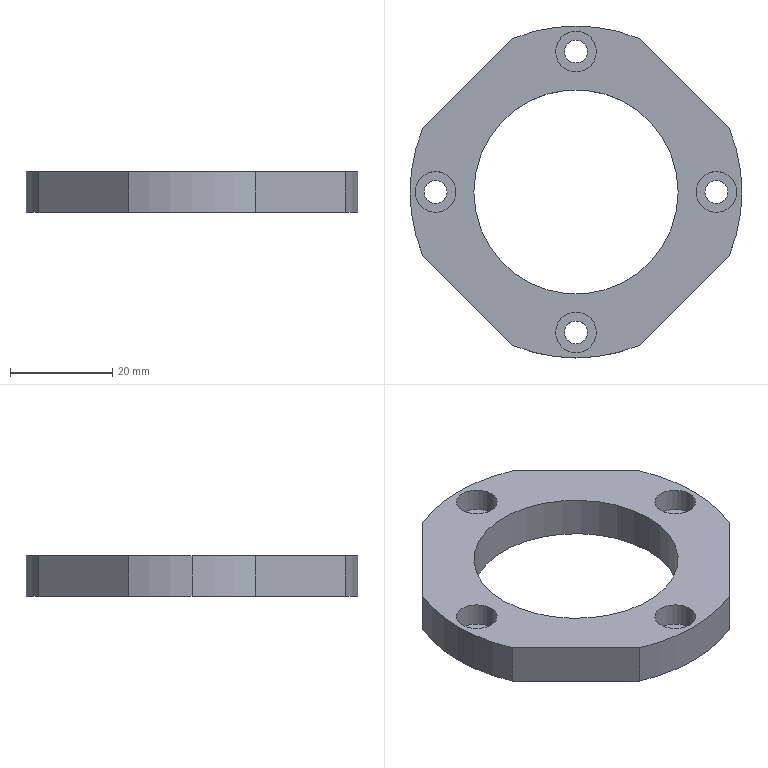Part | SolidWorks | features Extrusion 1, HoleWzd 1 | 1 solid | 33 faces | box 65 x 65 x 8 mm | volume 14008 mm3 | cylinder 23 | plane 10 | commonest cylinder face diameters 4.5 x8 8 x8 65 x5 40 x2
STEP:
#1=CARTESIAN_POINT('',(-4.,27.5,3.4));
#2=VERTEX_POINT('',#1);
#3=CARTESIAN_POINT('',(4.,27.5,3.4));
#4=VERTEX_POINT('',#3);
#5=CARTESIAN_POINT('',(0.,27.5,3.4));
#6=DIRECTION('',(0.,0.,1.));
#7=DIRECTION('',(1.,0.,0.));
#8=AXIS2_PLACEMENT_3D('',#5,#6,#7);
#9=CIRCLE('',#8,4.);
#10=EDGE_CURVE('',#2,#4,#9,.T.);
#11=ORIENTED_EDGE('',*,*,#10,.F.);
#12=CARTESIAN_POINT('',(-4.,27.5,8.));
#13=VERTEX_POINT('',#12);
#14=CARTESIAN_POINT('',(-4.,27.5,8.));
#15=DIRECTION('',(0.,0.,1.));
#16=VECTOR('',#15,1000.);
#17=LINE('',#14,#16);
#18=EDGE_CURVE('',#2,#13,#17,.T.);
#19=ORIENTED_EDGE('',*,*,#18,.T.);
#20=CARTESIAN_POINT('',(4.,27.5,8.));
#21=VERTEX_POINT('',#20);
#22=CARTESIAN_POINT('',(0.,27.5,8.));
#23=DIRECTION('',(0.,0.,1.));
#24=DIRECTION('',(1.,0.,0.));
#25=AXIS2_PLACEMENT_3D('',#22,#23,#24);
#26=CIRCLE('',#25,4.);
#27=EDGE_CURVE('',#13,#21,#26,.T.);
#28=ORIENTED_EDGE('',*,*,#27,.T.);
#29=CARTESIAN_POINT('',(4.,27.5,8.));
#30=DIRECTION('',(0.,0.,1.));
#31=VECTOR('',#30,1000.);
#32=LINE('',#29,#31);
#33=EDGE_CURVE('',#4,#21,#32,.T.);
#34=ORIENTED_EDGE('',*,*,#33,.F.);
#35=EDGE_LOOP('',(#11,#19,#28,#34));
#36=FACE_OUTER_BOUND('',#35,.T.);
#37=CARTESIAN_POINT('',(0.,27.5,8.));
#38=DIRECTION('',(0.,0.,1.));
#39=DIRECTION('',(1.,0.,0.));
#40=AXIS2_PLACEMENT_3D('',#37,#38,#39);
#41=CYLINDRICAL_SURFACE('',#40,4.);
#42=ADVANCED_FACE('',(#36),#41,.F.);
#43=CARTESIAN_POINT('',(-2.25,27.5,0.));
#44=VERTEX_POINT('',#43);
#45=CARTESIAN_POINT('',(2.25,27.5,0.));
#46=VERTEX_POINT('',#45);
#47=CARTESIAN_POINT('',(0.,27.5,0.));
#48=DIRECTION('',(0.,0.,1.));
#49=DIRECTION('',(1.,0.,0.));
#50=AXIS2_PLACEMENT_3D('',#47,#48,#49);
#51=CIRCLE('',#50,2.25);
#52=EDGE_CURVE('',#44,#46,#51,.T.);
#53=ORIENTED_EDGE('',*,*,#52,.F.);
#54=CARTESIAN_POINT('',(-2.25,27.5,3.4));
#55=VERTEX_POINT('',#54);
#56=CARTESIAN_POINT('',(-2.25,27.5,8.));
#57=DIRECTION('',(0.,0.,1.));
#58=VECTOR('',#57,1000.);
#59=LINE('',#56,#58);
#60=EDGE_CURVE('',#44,#55,#59,.T.);
#61=ORIENTED_EDGE('',*,*,#60,.T.);
#62=CARTESIAN_POINT('',(2.25,27.5,3.4));
#63=VERTEX_POINT('',#62);
#64=CARTESIAN_POINT('',(0.,27.5,3.4));
#65=DIRECTION('',(0.,0.,1.));
#66=DIRECTION('',(1.,0.,0.));
#67=AXIS2_PLACEMENT_3D('',#64,#65,#66);
#68=CIRCLE('',#67,2.25);
#69=EDGE_CURVE('',#55,#63,#68,.T.);
#70=ORIENTED_EDGE('',*,*,#69,.T.);
#71=CARTESIAN_POINT('',(2.25,27.5,8.));
#72=DIRECTION('',(0.,0.,1.));
#73=VECTOR('',#72,1000.);
#74=LINE('',#71,#73);
#75=EDGE_CURVE('',#46,#63,#74,.T.);
#76=ORIENTED_EDGE('',*,*,#75,.F.);
#77=EDGE_LOOP('',(#53,#61,#70,#76));
#78=FACE_OUTER_BOUND('',#77,.T.);
#79=CARTESIAN_POINT('',(0.,27.5,8.));
#80=DIRECTION('',(0.,0.,1.));
#81=DIRECTION('',(1.,0.,0.));
#82=AXIS2_PLACEMENT_3D('',#79,#80,#81);
#83=CYLINDRICAL_SURFACE('',#82,2.25);
#84=ADVANCED_FACE('',(#78),#83,.F.);
#85=CARTESIAN_POINT('',(-31.5,0.,3.4));
#86=VERTEX_POINT('',#85);
#87=CARTESIAN_POINT('',(-23.5,0.,3.4));
#88=VERTEX_POINT('',#87);
#89=CARTESIAN_POINT('',(-27.5,0.,3.4));
#90=DIRECTION('',(0.,0.,1.));
#91=DIRECTION('',(1.,0.,0.));
#92=AXIS2_PLACEMENT_3D('',#89,#90,#91);
#93=CIRCLE('',#92,4.);
#94=EDGE_CURVE('',#86,#88,#93,.T.);
#95=ORIENTED_EDGE('',*,*,#94,.F.);
#96=CARTESIAN_POINT('',(-31.5,0.,8.));
#97=VERTEX_POINT('',#96);
#98=CARTESIAN_POINT('',(-31.5,0.,8.));
#99=DIRECTION('',(0.,0.,1.));
#100=VECTOR('',#99,1000.);
#101=LINE('',#98,#100);
#102=EDGE_CURVE('',#86,#97,#101,.T.);
#103=ORIENTED_EDGE('',*,*,#102,.T.);
#104=CARTESIAN_POINT('',(-23.5,0.,8.));
#105=VERTEX_POINT('',#104);
#106=CARTESIAN_POINT('',(-27.5,0.,8.));
#107=DIRECTION('',(0.,0.,1.));
#108=DIRECTION('',(1.,0.,0.));
#109=AXIS2_PLACEMENT_3D('',#106,#107,#108);
#110=CIRCLE('',#109,4.);
#111=EDGE_CURVE('',#97,#105,#110,.T.);
#112=ORIENTED_EDGE('',*,*,#111,.T.);
#113=CARTESIAN_POINT('',(-23.5,0.,8.));
#114=DIRECTION('',(0.,0.,1.));
#115=VECTOR('',#114,1000.);
#116=LINE('',#113,#115);
#117=EDGE_CURVE('',#88,#105,#116,.T.);
#118=ORIENTED_EDGE('',*,*,#117,.F.);
#119=EDGE_LOOP('',(#95,#103,#112,#118));
#120=FACE_OUTER_BOUND('',#119,.T.);
#121=CARTESIAN_POINT('',(-27.5,0.,8.));
#122=DIRECTION('',(0.,0.,1.));
#123=DIRECTION('',(1.,0.,0.));
#124=AXIS2_PLACEMENT_3D('',#121,#122,#123);
#125=CYLINDRICAL_SURFACE('',#124,4.);
#126=ADVANCED_FACE('',(#120),#125,.F.);
#127=CARTESIAN_POINT('',(-29.75,0.,0.));
#128=VERTEX_POINT('',#127);
#129=CARTESIAN_POINT('',(-25.25,0.,0.));
#130=VERTEX_POINT('',#129);
#131=CARTESIAN_POINT('',(-27.5,0.,0.));
#132=DIRECTION('',(0.,0.,1.));
#133=DIRECTION('',(1.,0.,0.));
#134=AXIS2_PLACEMENT_3D('',#131,#132,#133);
#135=CIRCLE('',#134,2.25);
#136=EDGE_CURVE('',#128,#130,#135,.T.);
#137=ORIENTED_EDGE('',*,*,#136,.F.);
#138=CARTESIAN_POINT('',(-29.75,0.,3.4));
#139=VERTEX_POINT('',#138);
#140=CARTESIAN_POINT('',(-29.75,0.,8.));
#141=DIRECTION('',(0.,0.,1.));
#142=VECTOR('',#141,1000.);
#143=LINE('',#140,#142);
#144=EDGE_CURVE('',#128,#139,#143,.T.);
#145=ORIENTED_EDGE('',*,*,#144,.T.);
#146=CARTESIAN_POINT('',(-25.25,0.,3.4));
#147=VERTEX_POINT('',#146);
#148=CARTESIAN_POINT('',(-27.5,0.,3.4));
#149=DIRECTION('',(0.,0.,1.));
#150=DIRECTION('',(1.,0.,0.));
#151=AXIS2_PLACEMENT_3D('',#148,#149,#150);
#152=CIRCLE('',#151,2.25);
#153=EDGE_CURVE('',#139,#147,#152,.T.);
#154=ORIENTED_EDGE('',*,*,#153,.T.);
#155=CARTESIAN_POINT('',(-25.25,0.,8.));
#156=DIRECTION('',(0.,0.,1.));
#157=VECTOR('',#156,1000.);
#158=LINE('',#155,#157);
#159=EDGE_CURVE('',#130,#147,#158,.T.);
#160=ORIENTED_EDGE('',*,*,#159,.F.);
#161=EDGE_LOOP('',(#137,#145,#154,#160));
#162=FACE_OUTER_BOUND('',#161,.T.);
#163=CARTESIAN_POINT('',(-27.5,0.,8.));
#164=DIRECTION('',(0.,0.,1.));
#165=DIRECTION('',(1.,0.,0.));
#166=AXIS2_PLACEMENT_3D('',#163,#164,#165);
#167=CYLINDRICAL_SURFACE('',#166,2.25);
#168=ADVANCED_FACE('',(#162),#167,.F.);
#169=CARTESIAN_POINT('',(-4.,-27.5,3.4));
#170=VERTEX_POINT('',#169);
#171=CARTESIAN_POINT('',(4.,-27.5,3.4));
#172=VERTEX_POINT('',#171);
#173=CARTESIAN_POINT('',(0.,-27.5,3.4));
#174=DIRECTION('',(0.,0.,1.));
#175=DIRECTION('',(1.,0.,0.));
#176=AXIS2_PLACEMENT_3D('',#173,#174,#175);
#177=CIRCLE('',#176,4.);
#178=EDGE_CURVE('',#170,#172,#177,.T.);
#179=ORIENTED_EDGE('',*,*,#178,.F.);
#180=CARTESIAN_POINT('',(-4.,-27.5,8.));
#181=VERTEX_POINT('',#180);
#182=CARTESIAN_POINT('',(-4.,-27.5,8.));
#183=DIRECTION('',(0.,0.,1.));
#184=VECTOR('',#183,1000.);
#185=LINE('',#182,#184);
#186=EDGE_CURVE('',#170,#181,#185,.T.);
#187=ORIENTED_EDGE('',*,*,#186,.T.);
#188=CARTESIAN_POINT('',(4.,-27.5,8.));
#189=VERTEX_POINT('',#188);
#190=CARTESIAN_POINT('',(0.,-27.5,8.));
#191=DIRECTION('',(0.,0.,1.));
#192=DIRECTION('',(1.,0.,0.));
#193=AXIS2_PLACEMENT_3D('',#190,#191,#192);
#194=CIRCLE('',#193,4.);
#195=EDGE_CURVE('',#181,#189,#194,.T.);
#196=ORIENTED_EDGE('',*,*,#195,.T.);
#197=CARTESIAN_POINT('',(4.,-27.5,8.));
#198=DIRECTION('',(0.,0.,1.));
#199=VECTOR('',#198,1000.);
#200=LINE('',#197,#199);
#201=EDGE_CURVE('',#172,#189,#200,.T.);
#202=ORIENTED_EDGE('',*,*,#201,.F.);
#203=EDGE_LOOP('',(#179,#187,#196,#202));
#204=FACE_OUTER_BOUND('',#203,.T.);
#205=CARTESIAN_POINT('',(0.,-27.5,8.));
#206=DIRECTION('',(0.,0.,1.));
#207=DIRECTION('',(1.,0.,0.));
#208=AXIS2_PLACEMENT_3D('',#205,#206,#207);
#209=CYLINDRICAL_SURFACE('',#208,4.);
#210=ADVANCED_FACE('',(#204),#209,.F.);
#211=CARTESIAN_POINT('',(-2.25,-27.5,0.));
#212=VERTEX_POINT('',#211);
#213=CARTESIAN_POINT('',(2.25,-27.5,0.));
#214=VERTEX_POINT('',#213);
#215=CARTESIAN_POINT('',(0.,-27.5,0.));
#216=DIRECTION('',(0.,0.,1.));
#217=DIRECTION('',(1.,0.,0.));
#218=AXIS2_PLACEMENT_3D('',#215,#216,#217);
#219=CIRCLE('',#218,2.25);
#220=EDGE_CURVE('',#212,#214,#219,.T.);
#221=ORIENTED_EDGE('',*,*,#220,.F.);
#222=CARTESIAN_POINT('',(-2.25,-27.5,3.4));
#223=VERTEX_POINT('',#222);
#224=CARTESIAN_POINT('',(-2.25,-27.5,8.));
#225=DIRECTION('',(0.,0.,1.));
#226=VECTOR('',#225,1000.);
#227=LINE('',#224,#226);
#228=EDGE_CURVE('',#212,#223,#227,.T.);
#229=ORIENTED_EDGE('',*,*,#228,.T.);
#230=CARTESIAN_POINT('',(2.25,-27.5,3.4));
#231=VERTEX_POINT('',#230);
#232=CARTESIAN_POINT('',(0.,-27.5,3.4));
#233=DIRECTION('',(0.,0.,1.));
#234=DIRECTION('',(1.,0.,0.));
#235=AXIS2_PLACEMENT_3D('',#232,#233,#234);
#236=CIRCLE('',#235,2.25);
#237=EDGE_CURVE('',#223,#231,#236,.T.);
#238=ORIENTED_EDGE('',*,*,#237,.T.);
#239=CARTESIAN_POINT('',(2.25,-27.5,8.));
#240=DIRECTION('',(0.,0.,1.));
#241=VECTOR('',#240,1000.);
#242=LINE('',#239,#241);
#243=EDGE_CURVE('',#214,#231,#242,.T.);
#244=ORIENTED_EDGE('',*,*,#243,.F.);
#245=EDGE_LOOP('',(#221,#229,#238,#244));
#246=FACE_OUTER_BOUND('',#245,.T.);
#247=CARTESIAN_POINT('',(0.,-27.5,8.));
#248=DIRECTION('',(0.,0.,1.));
#249=DIRECTION('',(1.,0.,0.));
#250=AXIS2_PLACEMENT_3D('',#247,#248,#249);
#251=CYLINDRICAL_SURFACE('',#250,2.25);
#252=ADVANCED_FACE('',(#246),#251,.F.);
#253=CARTESIAN_POINT('',(23.5,0.,3.4));
#254=VERTEX_POINT('',#253);
#255=CARTESIAN_POINT('',(31.5,0.,3.4));
#256=VERTEX_POINT('',#255);
#257=CARTESIAN_POINT('',(27.5,0.,3.4));
#258=DIRECTION('',(0.,0.,1.));
#259=DIRECTION('',(1.,0.,0.));
#260=AXIS2_PLACEMENT_3D('',#257,#258,#259);
#261=CIRCLE('',#260,4.);
#262=EDGE_CURVE('',#254,#256,#261,.T.);
#263=ORIENTED_EDGE('',*,*,#262,.F.);
#264=CARTESIAN_POINT('',(23.5,0.,8.));
#265=VERTEX_POINT('',#264);
#266=CARTESIAN_POINT('',(23.5,0.,8.));
#267=DIRECTION('',(0.,0.,1.));
#268=VECTOR('',#267,1000.);
#269=LINE('',#266,#268);
#270=EDGE_CURVE('',#254,#265,#269,.T.);
#271=ORIENTED_EDGE('',*,*,#270,.T.);
#272=CARTESIAN_POINT('',(31.5,0.,8.));
#273=VERTEX_POINT('',#272);
#274=CARTESIAN_POINT('',(27.5,0.,8.));
#275=DIRECTION('',(0.,0.,1.));
#276=DIRECTION('',(1.,0.,0.));
#277=AXIS2_PLACEMENT_3D('',#274,#275,#276);
#278=CIRCLE('',#277,4.);
#279=EDGE_CURVE('',#265,#273,#278,.T.);
#280=ORIENTED_EDGE('',*,*,#279,.T.);
#281=CARTESIAN_POINT('',(31.5,0.,8.));
#282=DIRECTION('',(0.,0.,1.));
#283=VECTOR('',#282,1000.);
#284=LINE('',#281,#283);
#285=EDGE_CURVE('',#256,#273,#284,.T.);
#286=ORIENTED_EDGE('',*,*,#285,.F.);
#287=EDGE_LOOP('',(#263,#271,#280,#286));
#288=FACE_OUTER_BOUND('',#287,.T.);
#289=CARTESIAN_POINT('',(27.5,0.,8.));
#290=DIRECTION('',(0.,0.,1.));
#291=DIRECTION('',(1.,0.,0.));
#292=AXIS2_PLACEMENT_3D('',#289,#290,#291);
#293=CYLINDRICAL_SURFACE('',#292,4.);
#294=ADVANCED_FACE('',(#288),#293,.F.);
#295=CARTESIAN_POINT('',(25.25,0.,0.));
#296=VERTEX_POINT('',#295);
#297=CARTESIAN_POINT('',(29.75,0.,0.));
#298=VERTEX_POINT('',#297);
#299=CARTESIAN_POINT('',(27.5,0.,0.));
#300=DIRECTION('',(0.,0.,1.));
#301=DIRECTION('',(1.,0.,0.));
#302=AXIS2_PLACEMENT_3D('',#299,#300,#301);
#303=CIRCLE('',#302,2.25);
#304=EDGE_CURVE('',#296,#298,#303,.T.);
#305=ORIENTED_EDGE('',*,*,#304,.F.);
#306=CARTESIAN_POINT('',(25.25,0.,3.4));
#307=VERTEX_POINT('',#306);
#308=CARTESIAN_POINT('',(25.25,0.,8.));
#309=DIRECTION('',(0.,0.,1.));
#310=VECTOR('',#309,1000.);
#311=LINE('',#308,#310);
#312=EDGE_CURVE('',#296,#307,#311,.T.);
#313=ORIENTED_EDGE('',*,*,#312,.T.);
#314=CARTESIAN_POINT('',(29.75,0.,3.4));
#315=VERTEX_POINT('',#314);
#316=CARTESIAN_POINT('',(27.5,0.,3.4));
#317=DIRECTION('',(0.,0.,1.));
#318=DIRECTION('',(1.,0.,0.));
#319=AXIS2_PLACEMENT_3D('',#316,#317,#318);
#320=CIRCLE('',#319,2.25);
#321=EDGE_CURVE('',#307,#315,#320,.T.);
#322=ORIENTED_EDGE('',*,*,#321,.T.);
#323=CARTESIAN_POINT('',(29.75,0.,8.));
#324=DIRECTION('',(0.,0.,1.));
#325=VECTOR('',#324,1000.);
#326=LINE('',#323,#325);
#327=EDGE_CURVE('',#298,#315,#326,.T.);
#328=ORIENTED_EDGE('',*,*,#327,.F.);
#329=EDGE_LOOP('',(#305,#313,#322,#328));
#330=FACE_OUTER_BOUND('',#329,.T.);
#331=CARTESIAN_POINT('',(27.5,0.,8.));
#332=DIRECTION('',(0.,0.,1.));
#333=DIRECTION('',(1.,0.,0.));
#334=AXIS2_PLACEMENT_3D('',#331,#332,#333);
#335=CYLINDRICAL_SURFACE('',#334,2.25);
#336=ADVANCED_FACE('',(#330),#335,.F.);
#337=CARTESIAN_POINT('',(-20.,0.,8.));
#338=VERTEX_POINT('',#337);
#339=CARTESIAN_POINT('',(20.,0.,8.));
#340=VERTEX_POINT('',#339);
#341=CARTESIAN_POINT('',(0.,0.,8.));
#342=DIRECTION('',(0.,0.,1.));
#343=DIRECTION('',(1.,0.,0.));
#344=AXIS2_PLACEMENT_3D('',#341,#342,#343);
#345=CIRCLE('',#344,20.);
#346=EDGE_CURVE('',#338,#340,#345,.T.);
#347=ORIENTED_EDGE('',*,*,#346,.T.);
#348=CARTESIAN_POINT('',(20.,0.,0.));
#349=VERTEX_POINT('',#348);
#350=CARTESIAN_POINT('',(20.,0.,8.));
#351=DIRECTION('',(0.,0.,-1.));
#352=VECTOR('',#351,1000.);
#353=LINE('',#350,#352);
#354=EDGE_CURVE('',#340,#349,#353,.T.);
#355=ORIENTED_EDGE('',*,*,#354,.T.);
#356=CARTESIAN_POINT('',(-20.,0.,0.));
#357=VERTEX_POINT('',#356);
#358=CARTESIAN_POINT('',(0.,0.,0.));
#359=DIRECTION('',(0.,0.,1.));
#360=DIRECTION('',(1.,0.,0.));
#361=AXIS2_PLACEMENT_3D('',#358,#359,#360);
#362=CIRCLE('',#361,20.);
#363=EDGE_CURVE('',#357,#349,#362,.T.);
#364=ORIENTED_EDGE('',*,*,#363,.F.);
#365=CARTESIAN_POINT('',(-20.,0.,8.));
#366=DIRECTION('',(0.,0.,-1.));
#367=VECTOR('',#366,1000.);
#368=LINE('',#365,#367);
#369=EDGE_CURVE('',#338,#357,#368,.T.);
#370=ORIENTED_EDGE('',*,*,#369,.F.);
#371=EDGE_LOOP('',(#347,#355,#364,#370));
#372=FACE_OUTER_BOUND('',#371,.T.);
#373=CARTESIAN_POINT('',(0.,0.,8.));
#374=DIRECTION('',(0.,0.,-1.));
#375=DIRECTION('',(-1.,0.,0.));
#376=AXIS2_PLACEMENT_3D('',#373,#374,#375);
#377=CYLINDRICAL_SURFACE('',#376,20.);
#378=ADVANCED_FACE('',(#372),#377,.F.);
#379=CARTESIAN_POINT('',(-32.5,0.,8.));
#380=VERTEX_POINT('',#379);
#381=CARTESIAN_POINT('',(-30.052,-12.374,8.));
#382=VERTEX_POINT('',#381);
#383=CARTESIAN_POINT('',(0.,0.,8.));
#384=DIRECTION('',(0.,0.,1.));
#385=DIRECTION('',(1.,0.,0.));
#386=AXIS2_PLACEMENT_3D('',#383,#384,#385);
#387=CIRCLE('',#386,32.5);
#388=EDGE_CURVE('',#380,#382,#387,.T.);
#389=ORIENTED_EDGE('',*,*,#388,.F.);
#390=CARTESIAN_POINT('',(-32.5,0.,0.));
#391=VERTEX_POINT('',#390);
#392=CARTESIAN_POINT('',(-32.5,0.,8.));
#393=DIRECTION('',(0.,0.,-1.));
#394=VECTOR('',#393,1000.);
#395=LINE('',#392,#394);
#396=EDGE_CURVE('',#380,#391,#395,.T.);
#397=ORIENTED_EDGE('',*,*,#396,.T.);
#398=CARTESIAN_POINT('',(-30.052,-12.374,0.));
#399=VERTEX_POINT('',#398);
#400=CARTESIAN_POINT('',(0.,0.,0.));
#401=DIRECTION('',(0.,0.,1.));
#402=DIRECTION('',(1.,0.,0.));
#403=AXIS2_PLACEMENT_3D('',#400,#401,#402);
#404=CIRCLE('',#403,32.5);
#405=EDGE_CURVE('',#391,#399,#404,.T.);
#406=ORIENTED_EDGE('',*,*,#405,.T.);
#407=CARTESIAN_POINT('',(-30.052,-12.374,8.));
#408=DIRECTION('',(0.,0.,-1.));
#409=VECTOR('',#408,1000.);
#410=LINE('',#407,#409);
#411=EDGE_CURVE('',#382,#399,#410,.T.);
#412=ORIENTED_EDGE('',*,*,#411,.F.);
#413=EDGE_LOOP('',(#389,#397,#406,#412));
#414=FACE_OUTER_BOUND('',#413,.T.);
#415=CARTESIAN_POINT('',(0.,0.,8.));
#416=DIRECTION('',(0.,0.,-1.));
#417=DIRECTION('',(-1.,0.,0.));
#418=AXIS2_PLACEMENT_3D('',#415,#416,#417);
#419=CYLINDRICAL_SURFACE('',#418,32.5);
#420=ADVANCED_FACE('',(#414),#419,.T.);
#421=CARTESIAN_POINT('',(0.,27.5,8.));
#422=DIRECTION('',(0.,0.,1.));
#423=DIRECTION('',(1.,0.,0.));
#424=AXIS2_PLACEMENT_3D('',#421,#422,#423);
#425=CIRCLE('',#424,4.);
#426=EDGE_CURVE('',#21,#13,#425,.T.);
#427=ORIENTED_EDGE('',*,*,#426,.F.);
#428=ORIENTED_EDGE('',*,*,#27,.F.);
#429=EDGE_LOOP('',(#427,#428));
#430=FACE_BOUND('',#429,.T.);
#431=CARTESIAN_POINT('',(-27.5,0.,8.));
#432=DIRECTION('',(0.,0.,1.));
#433=DIRECTION('',(1.,0.,0.));
#434=AXIS2_PLACEMENT_3D('',#431,#432,#433);
#435=CIRCLE('',#434,4.);
#436=EDGE_CURVE('',#105,#97,#435,.T.);
#437=ORIENTED_EDGE('',*,*,#436,.F.);
#438=ORIENTED_EDGE('',*,*,#111,.F.);
#439=EDGE_LOOP('',(#437,#438));
#440=FACE_BOUND('',#439,.T.);
#441=CARTESIAN_POINT('',(0.,-27.5,8.));
#442=DIRECTION('',(0.,0.,1.));
#443=DIRECTION('',(1.,0.,0.));
#444=AXIS2_PLACEMENT_3D('',#441,#442,#443);
#445=CIRCLE('',#444,4.);
#446=EDGE_CURVE('',#189,#181,#445,.T.);
#447=ORIENTED_EDGE('',*,*,#446,.F.);
#448=ORIENTED_EDGE('',*,*,#195,.F.);
#449=EDGE_LOOP('',(#447,#448));
#450=FACE_BOUND('',#449,.T.);
#451=CARTESIAN_POINT('',(27.5,0.,8.));
#452=DIRECTION('',(0.,0.,1.));
#453=DIRECTION('',(1.,0.,0.));
#454=AXIS2_PLACEMENT_3D('',#451,#452,#453);
#455=CIRCLE('',#454,4.);
#456=EDGE_CURVE('',#273,#265,#455,.T.);
#457=ORIENTED_EDGE('',*,*,#456,.F.);
#458=ORIENTED_EDGE('',*,*,#279,.F.);
#459=EDGE_LOOP('',(#457,#458));
#460=FACE_BOUND('',#459,.T.);
#461=CARTESIAN_POINT('',(-30.052,12.374,8.));
#462=VERTEX_POINT('',#461);
#463=CARTESIAN_POINT('',(0.,0.,8.));
#464=DIRECTION('',(0.,0.,1.));
#465=DIRECTION('',(1.,0.,0.));
#466=AXIS2_PLACEMENT_3D('',#463,#464,#465);
#467=CIRCLE('',#466,32.5);
#468=EDGE_CURVE('',#462,#380,#467,.T.);
#469=ORIENTED_EDGE('',*,*,#468,.T.);
#470=ORIENTED_EDGE('',*,*,#388,.T.);
#471=CARTESIAN_POINT('',(-12.374,-30.052,8.));
#472=VERTEX_POINT('',#471);
#473=CARTESIAN_POINT('',(-30.052,-12.374,8.));
#474=DIRECTION('',(0.7071,-0.7071,0.));
#475=VECTOR('',#474,1000.);
#476=LINE('',#473,#475);
#477=EDGE_CURVE('',#382,#472,#476,.T.);
#478=ORIENTED_EDGE('',*,*,#477,.T.);
#479=CARTESIAN_POINT('',(12.374,-30.052,8.));
#480=VERTEX_POINT('',#479);
#481=CARTESIAN_POINT('',(0.,0.,8.));
#482=DIRECTION('',(0.,0.,1.));
#483=DIRECTION('',(1.,0.,0.));
#484=AXIS2_PLACEMENT_3D('',#481,#482,#483);
#485=CIRCLE('',#484,32.5);
#486=EDGE_CURVE('',#472,#480,#485,.T.);
#487=ORIENTED_EDGE('',*,*,#486,.T.);
#488=CARTESIAN_POINT('',(30.052,-12.374,8.));
#489=VERTEX_POINT('',#488);
#490=CARTESIAN_POINT('',(12.374,-30.052,8.));
#491=DIRECTION('',(0.7071,0.7071,0.));
#492=VECTOR('',#491,1000.);
#493=LINE('',#490,#492);
#494=EDGE_CURVE('',#480,#489,#493,.T.);
#495=ORIENTED_EDGE('',*,*,#494,.T.);
#496=CARTESIAN_POINT('',(30.052,12.374,8.));
#497=VERTEX_POINT('',#496);
#498=CARTESIAN_POINT('',(0.,0.,8.));
#499=DIRECTION('',(0.,0.,1.));
#500=DIRECTION('',(1.,0.,0.));
#501=AXIS2_PLACEMENT_3D('',#498,#499,#500);
#502=CIRCLE('',#501,32.5);
#503=EDGE_CURVE('',#489,#497,#502,.T.);
#504=ORIENTED_EDGE('',*,*,#503,.T.);
#505=CARTESIAN_POINT('',(12.374,30.052,8.));
#506=VERTEX_POINT('',#505);
#507=CARTESIAN_POINT('',(12.374,30.052,8.));
#508=DIRECTION('',(-0.7071,0.7071,0.));
#509=VECTOR('',#508,1000.);
#510=LINE('',#507,#509);
#511=EDGE_CURVE('',#497,#506,#510,.T.);
#512=ORIENTED_EDGE('',*,*,#511,.T.);
#513=CARTESIAN_POINT('',(-12.374,30.052,8.));
#514=VERTEX_POINT('',#513);
#515=CARTESIAN_POINT('',(0.,0.,8.));
#516=DIRECTION('',(0.,0.,1.));
#517=DIRECTION('',(1.,0.,0.));
#518=AXIS2_PLACEMENT_3D('',#515,#516,#517);
#519=CIRCLE('',#518,32.5);
#520=EDGE_CURVE('',#506,#514,#519,.T.);
#521=ORIENTED_EDGE('',*,*,#520,.T.);
#522=CARTESIAN_POINT('',(-30.052,12.374,8.));
#523=DIRECTION('',(-0.7071,-0.7071,0.));
#524=VECTOR('',#523,1000.);
#525=LINE('',#522,#524);
#526=EDGE_CURVE('',#514,#462,#525,.T.);
#527=ORIENTED_EDGE('',*,*,#526,.T.);
#528=EDGE_LOOP('',(#469,#470,#478,#487,#495,#504,#512,#521,#527));
#529=FACE_OUTER_BOUND('',#528,.T.);
#530=ORIENTED_EDGE('',*,*,#346,.F.);
#531=CARTESIAN_POINT('',(0.,0.,8.));
#532=DIRECTION('',(0.,0.,1.));
#533=DIRECTION('',(1.,0.,0.));
#534=AXIS2_PLACEMENT_3D('',#531,#532,#533);
#535=CIRCLE('',#534,20.);
#536=EDGE_CURVE('',#340,#338,#535,.T.);
#537=ORIENTED_EDGE('',*,*,#536,.F.);
#538=EDGE_LOOP('',(#530,#537));
#539=FACE_BOUND('',#538,.T.);
#540=CARTESIAN_POINT('',(0.,0.,8.));
#541=DIRECTION('',(0.,0.,1.));
#542=DIRECTION('',(1.,0.,0.));
#543=AXIS2_PLACEMENT_3D('',#540,#541,#542);
#544=PLANE('',#543);
#545=ADVANCED_FACE('',(#430,#440,#450,#460,#529,#539),#544,.T.);
#546=CARTESIAN_POINT('',(0.,27.5,0.));
#547=DIRECTION('',(0.,0.,1.));
#548=DIRECTION('',(1.,0.,0.));
#549=AXIS2_PLACEMENT_3D('',#546,#547,#548);
#550=CIRCLE('',#549,2.25);
#551=EDGE_CURVE('',#46,#44,#550,.T.);
#552=ORIENTED_EDGE('',*,*,#551,.T.);
#553=ORIENTED_EDGE('',*,*,#52,.T.);
#554=EDGE_LOOP('',(#552,#553));
#555=FACE_BOUND('',#554,.T.);
#556=CARTESIAN_POINT('',(-27.5,0.,0.));
#557=DIRECTION('',(0.,0.,1.));
#558=DIRECTION('',(1.,0.,0.));
#559=AXIS2_PLACEMENT_3D('',#556,#557,#558);
#560=CIRCLE('',#559,2.25);
#561=EDGE_CURVE('',#130,#128,#560,.T.);
#562=ORIENTED_EDGE('',*,*,#561,.T.);
#563=ORIENTED_EDGE('',*,*,#136,.T.);
#564=EDGE_LOOP('',(#562,#563));
#565=FACE_BOUND('',#564,.T.);
#566=CARTESIAN_POINT('',(0.,-27.5,0.));
#567=DIRECTION('',(0.,0.,1.));
#568=DIRECTION('',(1.,0.,0.));
#569=AXIS2_PLACEMENT_3D('',#566,#567,#568);
#570=CIRCLE('',#569,2.25);
#571=EDGE_CURVE('',#214,#212,#570,.T.);
#572=ORIENTED_EDGE('',*,*,#571,.T.);
#573=ORIENTED_EDGE('',*,*,#220,.T.);
#574=EDGE_LOOP('',(#572,#573));
#575=FACE_BOUND('',#574,.T.);
#576=CARTESIAN_POINT('',(27.5,0.,0.));
#577=DIRECTION('',(0.,0.,1.));
#578=DIRECTION('',(1.,0.,0.));
#579=AXIS2_PLACEMENT_3D('',#576,#577,#578);
#580=CIRCLE('',#579,2.25);
#581=EDGE_CURVE('',#298,#296,#580,.T.);
#582=ORIENTED_EDGE('',*,*,#581,.T.);
#583=ORIENTED_EDGE('',*,*,#304,.T.);
#584=EDGE_LOOP('',(#582,#583));
#585=FACE_BOUND('',#584,.T.);
#586=CARTESIAN_POINT('',(-30.052,12.374,0.));
#587=VERTEX_POINT('',#586);
#588=CARTESIAN_POINT('',(0.,0.,0.));
#589=DIRECTION('',(0.,0.,1.));
#590=DIRECTION('',(1.,0.,0.));
#591=AXIS2_PLACEMENT_3D('',#588,#589,#590);
#592=CIRCLE('',#591,32.5);
#593=EDGE_CURVE('',#587,#391,#592,.T.);
#594=ORIENTED_EDGE('',*,*,#593,.F.);
#595=CARTESIAN_POINT('',(-12.374,30.052,0.));
#596=VERTEX_POINT('',#595);
#597=CARTESIAN_POINT('',(-30.052,12.374,0.));
#598=DIRECTION('',(-0.7071,-0.7071,0.));
#599=VECTOR('',#598,1000.);
#600=LINE('',#597,#599);
#601=EDGE_CURVE('',#596,#587,#600,.T.);
#602=ORIENTED_EDGE('',*,*,#601,.F.);
#603=CARTESIAN_POINT('',(12.374,30.052,0.));
#604=VERTEX_POINT('',#603);
#605=CARTESIAN_POINT('',(0.,0.,0.));
#606=DIRECTION('',(0.,0.,1.));
#607=DIRECTION('',(1.,0.,0.));
#608=AXIS2_PLACEMENT_3D('',#605,#606,#607);
#609=CIRCLE('',#608,32.5);
#610=EDGE_CURVE('',#604,#596,#609,.T.);
#611=ORIENTED_EDGE('',*,*,#610,.F.);
#612=CARTESIAN_POINT('',(30.052,12.374,0.));
#613=VERTEX_POINT('',#612);
#614=CARTESIAN_POINT('',(12.374,30.052,0.));
#615=DIRECTION('',(-0.7071,0.7071,0.));
#616=VECTOR('',#615,1000.);
#617=LINE('',#614,#616);
#618=EDGE_CURVE('',#613,#604,#617,.T.);
#619=ORIENTED_EDGE('',*,*,#618,.F.);
#620=CARTESIAN_POINT('',(30.052,-12.374,0.));
#621=VERTEX_POINT('',#620);
#622=CARTESIAN_POINT('',(0.,0.,0.));
#623=DIRECTION('',(0.,0.,1.));
#624=DIRECTION('',(1.,0.,0.));
#625=AXIS2_PLACEMENT_3D('',#622,#623,#624);
#626=CIRCLE('',#625,32.5);
#627=EDGE_CURVE('',#621,#613,#626,.T.);
#628=ORIENTED_EDGE('',*,*,#627,.F.);
#629=CARTESIAN_POINT('',(12.374,-30.052,0.));
#630=VERTEX_POINT('',#629);
#631=CARTESIAN_POINT('',(12.374,-30.052,0.));
#632=DIRECTION('',(0.7071,0.7071,0.));
#633=VECTOR('',#632,1000.);
#634=LINE('',#631,#633);
#635=EDGE_CURVE('',#630,#621,#634,.T.);
#636=ORIENTED_EDGE('',*,*,#635,.F.);
#637=CARTESIAN_POINT('',(-12.374,-30.052,0.));
#638=VERTEX_POINT('',#637);
#639=CARTESIAN_POINT('',(0.,0.,0.));
#640=DIRECTION('',(0.,0.,1.));
#641=DIRECTION('',(1.,0.,0.));
#642=AXIS2_PLACEMENT_3D('',#639,#640,#641);
#643=CIRCLE('',#642,32.5);
#644=EDGE_CURVE('',#638,#630,#643,.T.);
#645=ORIENTED_EDGE('',*,*,#644,.F.);
#646=CARTESIAN_POINT('',(-30.052,-12.374,0.));
#647=DIRECTION('',(0.7071,-0.7071,0.));
#648=VECTOR('',#647,1000.);
#649=LINE('',#646,#648);
#650=EDGE_CURVE('',#399,#638,#649,.T.);
#651=ORIENTED_EDGE('',*,*,#650,.F.);
#652=ORIENTED_EDGE('',*,*,#405,.F.);
#653=EDGE_LOOP('',(#594,#602,#611,#619,#628,#636,#645,#651,#652));
#654=FACE_OUTER_BOUND('',#653,.T.);
#655=ORIENTED_EDGE('',*,*,#363,.T.);
#656=CARTESIAN_POINT('',(0.,0.,0.));
#657=DIRECTION('',(0.,0.,1.));
#658=DIRECTION('',(1.,0.,0.));
#659=AXIS2_PLACEMENT_3D('',#656,#657,#658);
#660=CIRCLE('',#659,20.);
#661=EDGE_CURVE('',#349,#357,#660,.T.);
#662=ORIENTED_EDGE('',*,*,#661,.T.);
#663=EDGE_LOOP('',(#655,#662));
#664=FACE_BOUND('',#663,.T.);
#665=CARTESIAN_POINT('',(0.,0.,0.));
#666=DIRECTION('',(0.,0.,1.));
#667=DIRECTION('',(1.,0.,0.));
#668=AXIS2_PLACEMENT_3D('',#665,#666,#667);
#669=PLANE('',#668);
#670=ADVANCED_FACE('',(#555,#565,#575,#585,#654,#664),#669,.F.);
#671=ORIENTED_EDGE('',*,*,#396,.F.);
#672=ORIENTED_EDGE('',*,*,#468,.F.);
#673=CARTESIAN_POINT('',(-30.052,12.374,8.));
#674=DIRECTION('',(0.,0.,-1.));
#675=VECTOR('',#674,1000.);
#676=LINE('',#673,#675);
#677=EDGE_CURVE('',#462,#587,#676,.T.);
#678=ORIENTED_EDGE('',*,*,#677,.T.);
#679=ORIENTED_EDGE('',*,*,#593,.T.);
#680=EDGE_LOOP('',(#671,#672,#678,#679));
#681=FACE_OUTER_BOUND('',#680,.T.);
#682=CARTESIAN_POINT('',(0.,0.,8.));
#683=DIRECTION('',(0.,0.,-1.));
#684=DIRECTION('',(-1.,0.,0.));
#685=AXIS2_PLACEMENT_3D('',#682,#683,#684);
#686=CYLINDRICAL_SURFACE('',#685,32.5);
#687=ADVANCED_FACE('',(#681),#686,.T.);
#688=ORIENTED_EDGE('',*,*,#650,.T.);
#689=CARTESIAN_POINT('',(-12.374,-30.052,8.));
#690=DIRECTION('',(0.,0.,-1.));
#691=VECTOR('',#690,1000.);
#692=LINE('',#689,#691);
#693=EDGE_CURVE('',#472,#638,#692,.T.);
#694=ORIENTED_EDGE('',*,*,#693,.F.);
#695=ORIENTED_EDGE('',*,*,#477,.F.);
#696=ORIENTED_EDGE('',*,*,#411,.T.);
#697=EDGE_LOOP('',(#688,#694,#695,#696));
#698=FACE_OUTER_BOUND('',#697,.T.);
#699=CARTESIAN_POINT('',(-30.052,-12.374,8.));
#700=DIRECTION('',(0.7071,0.7071,0.));
#701=DIRECTION('',(-0.7071,0.7071,0.));
#702=AXIS2_PLACEMENT_3D('',#699,#700,#701);
#703=PLANE('',#702);
#704=ADVANCED_FACE('',(#698),#703,.F.);
#705=ORIENTED_EDGE('',*,*,#644,.T.);
#706=CARTESIAN_POINT('',(12.374,-30.052,8.));
#707=DIRECTION('',(0.,0.,-1.));
#708=VECTOR('',#707,1000.);
#709=LINE('',#706,#708);
#710=EDGE_CURVE('',#480,#630,#709,.T.);
#711=ORIENTED_EDGE('',*,*,#710,.F.);
#712=ORIENTED_EDGE('',*,*,#486,.F.);
#713=ORIENTED_EDGE('',*,*,#693,.T.);
#714=EDGE_LOOP('',(#705,#711,#712,#713));
#715=FACE_OUTER_BOUND('',#714,.T.);
#716=CARTESIAN_POINT('',(0.,0.,8.));
#717=DIRECTION('',(0.,0.,-1.));
#718=DIRECTION('',(-1.,0.,0.));
#719=AXIS2_PLACEMENT_3D('',#716,#717,#718);
#720=CYLINDRICAL_SURFACE('',#719,32.5);
#721=ADVANCED_FACE('',(#715),#720,.T.);
#722=ORIENTED_EDGE('',*,*,#635,.T.);
#723=CARTESIAN_POINT('',(30.052,-12.374,8.));
#724=DIRECTION('',(0.,0.,-1.));
#725=VECTOR('',#724,1000.);
#726=LINE('',#723,#725);
#727=EDGE_CURVE('',#489,#621,#726,.T.);
#728=ORIENTED_EDGE('',*,*,#727,.F.);
#729=ORIENTED_EDGE('',*,*,#494,.F.);
#730=ORIENTED_EDGE('',*,*,#710,.T.);
#731=EDGE_LOOP('',(#722,#728,#729,#730));
#732=FACE_OUTER_BOUND('',#731,.T.);
#733=CARTESIAN_POINT('',(12.374,-30.052,8.));
#734=DIRECTION('',(-0.7071,0.7071,0.));
#735=DIRECTION('',(-0.7071,-0.7071,0.));
#736=AXIS2_PLACEMENT_3D('',#733,#734,#735);
#737=PLANE('',#736);
#738=ADVANCED_FACE('',(#732),#737,.F.);
#739=ORIENTED_EDGE('',*,*,#627,.T.);
#740=CARTESIAN_POINT('',(30.052,12.374,8.));
#741=DIRECTION('',(0.,0.,-1.));
#742=VECTOR('',#741,1000.);
#743=LINE('',#740,#742);
#744=EDGE_CURVE('',#497,#613,#743,.T.);
#745=ORIENTED_EDGE('',*,*,#744,.F.);
#746=ORIENTED_EDGE('',*,*,#503,.F.);
#747=ORIENTED_EDGE('',*,*,#727,.T.);
#748=EDGE_LOOP('',(#739,#745,#746,#747));
#749=FACE_OUTER_BOUND('',#748,.T.);
#750=CARTESIAN_POINT('',(0.,0.,8.));
#751=DIRECTION('',(0.,0.,-1.));
#752=DIRECTION('',(-1.,0.,0.));
#753=AXIS2_PLACEMENT_3D('',#750,#751,#752);
#754=CYLINDRICAL_SURFACE('',#753,32.5);
#755=ADVANCED_FACE('',(#749),#754,.T.);
#756=ORIENTED_EDGE('',*,*,#618,.T.);
#757=CARTESIAN_POINT('',(12.374,30.052,8.));
#758=DIRECTION('',(0.,0.,-1.));
#759=VECTOR('',#758,1000.);
#760=LINE('',#757,#759);
#761=EDGE_CURVE('',#506,#604,#760,.T.);
#762=ORIENTED_EDGE('',*,*,#761,.F.);
#763=ORIENTED_EDGE('',*,*,#511,.F.);
#764=ORIENTED_EDGE('',*,*,#744,.T.);
#765=EDGE_LOOP('',(#756,#762,#763,#764));
#766=FACE_OUTER_BOUND('',#765,.T.);
#767=CARTESIAN_POINT('',(12.374,30.052,8.));
#768=DIRECTION('',(-0.7071,-0.7071,0.));
#769=DIRECTION('',(0.7071,-0.7071,0.));
#770=AXIS2_PLACEMENT_3D('',#767,#768,#769);
#771=PLANE('',#770);
#772=ADVANCED_FACE('',(#766),#771,.F.);
#773=ORIENTED_EDGE('',*,*,#610,.T.);
#774=CARTESIAN_POINT('',(-12.374,30.052,8.));
#775=DIRECTION('',(0.,0.,-1.));
#776=VECTOR('',#775,1000.);
#777=LINE('',#774,#776);
#778=EDGE_CURVE('',#514,#596,#777,.T.);
#779=ORIENTED_EDGE('',*,*,#778,.F.);
#780=ORIENTED_EDGE('',*,*,#520,.F.);
#781=ORIENTED_EDGE('',*,*,#761,.T.);
#782=EDGE_LOOP('',(#773,#779,#780,#781));
#783=FACE_OUTER_BOUND('',#782,.T.);
#784=CARTESIAN_POINT('',(0.,0.,8.));
#785=DIRECTION('',(0.,0.,-1.));
#786=DIRECTION('',(-1.,0.,0.));
#787=AXIS2_PLACEMENT_3D('',#784,#785,#786);
#788=CYLINDRICAL_SURFACE('',#787,32.5);
#789=ADVANCED_FACE('',(#783),#788,.T.);
#790=ORIENTED_EDGE('',*,*,#601,.T.);
#791=ORIENTED_EDGE('',*,*,#677,.F.);
#792=ORIENTED_EDGE('',*,*,#526,.F.);
#793=ORIENTED_EDGE('',*,*,#778,.T.);
#794=EDGE_LOOP('',(#790,#791,#792,#793));
#795=FACE_OUTER_BOUND('',#794,.T.);
#796=CARTESIAN_POINT('',(-30.052,12.374,8.));
#797=DIRECTION('',(0.7071,-0.7071,0.));
#798=DIRECTION('',(0.7071,0.7071,0.));
#799=AXIS2_PLACEMENT_3D('',#796,#797,#798);
#800=PLANE('',#799);
#801=ADVANCED_FACE('',(#795),#800,.F.);
#802=ORIENTED_EDGE('',*,*,#354,.F.);
#803=ORIENTED_EDGE('',*,*,#536,.T.);
#804=ORIENTED_EDGE('',*,*,#369,.T.);
#805=ORIENTED_EDGE('',*,*,#661,.F.);
#806=EDGE_LOOP('',(#802,#803,#804,#805));
#807=FACE_OUTER_BOUND('',#806,.T.);
#808=CARTESIAN_POINT('',(0.,0.,8.));
#809=DIRECTION('',(0.,0.,-1.));
#810=DIRECTION('',(-1.,0.,0.));
#811=AXIS2_PLACEMENT_3D('',#808,#809,#810);
#812=CYLINDRICAL_SURFACE('',#811,20.);
#813=ADVANCED_FACE('',(#807),#812,.F.);
#814=ORIENTED_EDGE('',*,*,#312,.F.);
#815=ORIENTED_EDGE('',*,*,#581,.F.);
#816=ORIENTED_EDGE('',*,*,#327,.T.);
#817=CARTESIAN_POINT('',(27.5,0.,3.4));
#818=DIRECTION('',(0.,0.,1.));
#819=DIRECTION('',(1.,0.,0.));
#820=AXIS2_PLACEMENT_3D('',#817,#818,#819);
#821=CIRCLE('',#820,2.25);
#822=EDGE_CURVE('',#315,#307,#821,.T.);
#823=ORIENTED_EDGE('',*,*,#822,.T.);
#824=EDGE_LOOP('',(#814,#815,#816,#823));
#825=FACE_OUTER_BOUND('',#824,.T.);
#826=CARTESIAN_POINT('',(27.5,0.,8.));
#827=DIRECTION('',(0.,0.,1.));
#828=DIRECTION('',(1.,0.,0.));
#829=AXIS2_PLACEMENT_3D('',#826,#827,#828);
#830=CYLINDRICAL_SURFACE('',#829,2.25);
#831=ADVANCED_FACE('',(#825),#830,.F.);
#832=ORIENTED_EDGE('',*,*,#822,.F.);
#833=ORIENTED_EDGE('',*,*,#321,.F.);
#834=EDGE_LOOP('',(#832,#833));
#835=FACE_BOUND('',#834,.T.);
#836=CARTESIAN_POINT('',(27.5,0.,3.4));
#837=DIRECTION('',(0.,0.,1.));
#838=DIRECTION('',(1.,0.,0.));
#839=AXIS2_PLACEMENT_3D('',#836,#837,#838);
#840=CIRCLE('',#839,4.);
#841=EDGE_CURVE('',#256,#254,#840,.T.);
#842=ORIENTED_EDGE('',*,*,#841,.T.);
#843=ORIENTED_EDGE('',*,*,#262,.T.);
#844=EDGE_LOOP('',(#842,#843));
#845=FACE_OUTER_BOUND('',#844,.T.);
#846=CARTESIAN_POINT('',(29.75,0.,3.4));
#847=DIRECTION('',(0.,0.,-1.));
#848=DIRECTION('',(-1.,0.,0.));
#849=AXIS2_PLACEMENT_3D('',#846,#847,#848);
#850=PLANE('',#849);
#851=ADVANCED_FACE('',(#835,#845),#850,.F.);
#852=ORIENTED_EDGE('',*,*,#270,.F.);
#853=ORIENTED_EDGE('',*,*,#841,.F.);
#854=ORIENTED_EDGE('',*,*,#285,.T.);
#855=ORIENTED_EDGE('',*,*,#456,.T.);
#856=EDGE_LOOP('',(#852,#853,#854,#855));
#857=FACE_OUTER_BOUND('',#856,.T.);
#858=CARTESIAN_POINT('',(27.5,0.,8.));
#859=DIRECTION('',(0.,0.,1.));
#860=DIRECTION('',(1.,0.,0.));
#861=AXIS2_PLACEMENT_3D('',#858,#859,#860);
#862=CYLINDRICAL_SURFACE('',#861,4.);
#863=ADVANCED_FACE('',(#857),#862,.F.);
#864=ORIENTED_EDGE('',*,*,#228,.F.);
#865=ORIENTED_EDGE('',*,*,#571,.F.);
#866=ORIENTED_EDGE('',*,*,#243,.T.);
#867=CARTESIAN_POINT('',(0.,-27.5,3.4));
#868=DIRECTION('',(0.,0.,1.));
#869=DIRECTION('',(1.,0.,0.));
#870=AXIS2_PLACEMENT_3D('',#867,#868,#869);
#871=CIRCLE('',#870,2.25);
#872=EDGE_CURVE('',#231,#223,#871,.T.);
#873=ORIENTED_EDGE('',*,*,#872,.T.);
#874=EDGE_LOOP('',(#864,#865,#866,#873));
#875=FACE_OUTER_BOUND('',#874,.T.);
#876=CARTESIAN_POINT('',(0.,-27.5,8.));
#877=DIRECTION('',(0.,0.,1.));
#878=DIRECTION('',(1.,0.,0.));
#879=AXIS2_PLACEMENT_3D('',#876,#877,#878);
#880=CYLINDRICAL_SURFACE('',#879,2.25);
#881=ADVANCED_FACE('',(#875),#880,.F.);
#882=ORIENTED_EDGE('',*,*,#872,.F.);
#883=ORIENTED_EDGE('',*,*,#237,.F.);
#884=EDGE_LOOP('',(#882,#883));
#885=FACE_BOUND('',#884,.T.);
#886=CARTESIAN_POINT('',(0.,-27.5,3.4));
#887=DIRECTION('',(0.,0.,1.));
#888=DIRECTION('',(1.,0.,0.));
#889=AXIS2_PLACEMENT_3D('',#886,#887,#888);
#890=CIRCLE('',#889,4.);
#891=EDGE_CURVE('',#172,#170,#890,.T.);
#892=ORIENTED_EDGE('',*,*,#891,.T.);
#893=ORIENTED_EDGE('',*,*,#178,.T.);
#894=EDGE_LOOP('',(#892,#893));
#895=FACE_OUTER_BOUND('',#894,.T.);
#896=CARTESIAN_POINT('',(2.25,-27.5,3.4));
#897=DIRECTION('',(0.,0.,-1.));
#898=DIRECTION('',(-1.,0.,0.));
#899=AXIS2_PLACEMENT_3D('',#896,#897,#898);
#900=PLANE('',#899);
#901=ADVANCED_FACE('',(#885,#895),#900,.F.);
#902=ORIENTED_EDGE('',*,*,#186,.F.);
#903=ORIENTED_EDGE('',*,*,#891,.F.);
#904=ORIENTED_EDGE('',*,*,#201,.T.);
#905=ORIENTED_EDGE('',*,*,#446,.T.);
#906=EDGE_LOOP('',(#902,#903,#904,#905));
#907=FACE_OUTER_BOUND('',#906,.T.);
#908=CARTESIAN_POINT('',(0.,-27.5,8.));
#909=DIRECTION('',(0.,0.,1.));
#910=DIRECTION('',(1.,0.,0.));
#911=AXIS2_PLACEMENT_3D('',#908,#909,#910);
#912=CYLINDRICAL_SURFACE('',#911,4.);
#913=ADVANCED_FACE('',(#907),#912,.F.);
#914=ORIENTED_EDGE('',*,*,#144,.F.);
#915=ORIENTED_EDGE('',*,*,#561,.F.);
#916=ORIENTED_EDGE('',*,*,#159,.T.);
#917=CARTESIAN_POINT('',(-27.5,0.,3.4));
#918=DIRECTION('',(0.,0.,1.));
#919=DIRECTION('',(1.,0.,0.));
#920=AXIS2_PLACEMENT_3D('',#917,#918,#919);
#921=CIRCLE('',#920,2.25);
#922=EDGE_CURVE('',#147,#139,#921,.T.);
#923=ORIENTED_EDGE('',*,*,#922,.T.);
#924=EDGE_LOOP('',(#914,#915,#916,#923));
#925=FACE_OUTER_BOUND('',#924,.T.);
#926=CARTESIAN_POINT('',(-27.5,0.,8.));
#927=DIRECTION('',(0.,0.,1.));
#928=DIRECTION('',(1.,0.,0.));
#929=AXIS2_PLACEMENT_3D('',#926,#927,#928);
#930=CYLINDRICAL_SURFACE('',#929,2.25);
#931=ADVANCED_FACE('',(#925),#930,.F.);
#932=ORIENTED_EDGE('',*,*,#922,.F.);
#933=ORIENTED_EDGE('',*,*,#153,.F.);
#934=EDGE_LOOP('',(#932,#933));
#935=FACE_BOUND('',#934,.T.);
#936=CARTESIAN_POINT('',(-27.5,0.,3.4));
#937=DIRECTION('',(0.,0.,1.));
#938=DIRECTION('',(1.,0.,0.));
#939=AXIS2_PLACEMENT_3D('',#936,#937,#938);
#940=CIRCLE('',#939,4.);
#941=EDGE_CURVE('',#88,#86,#940,.T.);
#942=ORIENTED_EDGE('',*,*,#941,.T.);
#943=ORIENTED_EDGE('',*,*,#94,.T.);
#944=EDGE_LOOP('',(#942,#943));
#945=FACE_OUTER_BOUND('',#944,.T.);
#946=CARTESIAN_POINT('',(-25.25,0.,3.4));
#947=DIRECTION('',(0.,0.,-1.));
#948=DIRECTION('',(-1.,0.,0.));
#949=AXIS2_PLACEMENT_3D('',#946,#947,#948);
#950=PLANE('',#949);
#951=ADVANCED_FACE('',(#935,#945),#950,.F.);
#952=ORIENTED_EDGE('',*,*,#102,.F.);
#953=ORIENTED_EDGE('',*,*,#941,.F.);
#954=ORIENTED_EDGE('',*,*,#117,.T.);
#955=ORIENTED_EDGE('',*,*,#436,.T.);
#956=EDGE_LOOP('',(#952,#953,#954,#955));
#957=FACE_OUTER_BOUND('',#956,.T.);
#958=CARTESIAN_POINT('',(-27.5,0.,8.));
#959=DIRECTION('',(0.,0.,1.));
#960=DIRECTION('',(1.,0.,0.));
#961=AXIS2_PLACEMENT_3D('',#958,#959,#960);
#962=CYLINDRICAL_SURFACE('',#961,4.);
#963=ADVANCED_FACE('',(#957),#962,.F.);
#964=ORIENTED_EDGE('',*,*,#60,.F.);
#965=ORIENTED_EDGE('',*,*,#551,.F.);
#966=ORIENTED_EDGE('',*,*,#75,.T.);
#967=CARTESIAN_POINT('',(0.,27.5,3.4));
#968=DIRECTION('',(0.,0.,1.));
#969=DIRECTION('',(1.,0.,0.));
#970=AXIS2_PLACEMENT_3D('',#967,#968,#969);
#971=CIRCLE('',#970,2.25);
#972=EDGE_CURVE('',#63,#55,#971,.T.);
#973=ORIENTED_EDGE('',*,*,#972,.T.);
#974=EDGE_LOOP('',(#964,#965,#966,#973));
#975=FACE_OUTER_BOUND('',#974,.T.);
#976=CARTESIAN_POINT('',(0.,27.5,8.));
#977=DIRECTION('',(0.,0.,1.));
#978=DIRECTION('',(1.,0.,0.));
#979=AXIS2_PLACEMENT_3D('',#976,#977,#978);
#980=CYLINDRICAL_SURFACE('',#979,2.25);
#981=ADVANCED_FACE('',(#975),#980,.F.);
#982=ORIENTED_EDGE('',*,*,#972,.F.);
#983=ORIENTED_EDGE('',*,*,#69,.F.);
#984=EDGE_LOOP('',(#982,#983));
#985=FACE_BOUND('',#984,.T.);
#986=CARTESIAN_POINT('',(0.,27.5,3.4));
#987=DIRECTION('',(0.,0.,1.));
#988=DIRECTION('',(1.,0.,0.));
#989=AXIS2_PLACEMENT_3D('',#986,#987,#988);
#990=CIRCLE('',#989,4.);
#991=EDGE_CURVE('',#4,#2,#990,.T.);
#992=ORIENTED_EDGE('',*,*,#991,.T.);
#993=ORIENTED_EDGE('',*,*,#10,.T.);
#994=EDGE_LOOP('',(#992,#993));
#995=FACE_OUTER_BOUND('',#994,.T.);
#996=CARTESIAN_POINT('',(2.25,27.5,3.4));
#997=DIRECTION('',(0.,0.,-1.));
#998=DIRECTION('',(-1.,0.,0.));
#999=AXIS2_PLACEMENT_3D('',#996,#997,#998);
#1000=PLANE('',#999);
#1001=ADVANCED_FACE('',(#985,#995),#1000,.F.);
#1002=ORIENTED_EDGE('',*,*,#18,.F.);
#1003=ORIENTED_EDGE('',*,*,#991,.F.);
#1004=ORIENTED_EDGE('',*,*,#33,.T.);
#1005=ORIENTED_EDGE('',*,*,#426,.T.);
#1006=EDGE_LOOP('',(#1002,#1003,#1004,#1005));
#1007=FACE_OUTER_BOUND('',#1006,.T.);
#1008=CARTESIAN_POINT('',(0.,27.5,8.));
#1009=DIRECTION('',(0.,0.,1.));
#1010=DIRECTION('',(1.,0.,0.));
#1011=AXIS2_PLACEMENT_3D('',#1008,#1009,#1010);
#1012=CYLINDRICAL_SURFACE('',#1011,4.);
#1013=ADVANCED_FACE('',(#1007),#1012,.F.);
#1014=CLOSED_SHELL('',(#42,#84,#126,#168,#210,#252,#294,#336,#378,#420,#545,#670,#687,#704,#721,#738,#755,#772,#789,#801,#813,#831,#851,#863,#881,#901,#913,#931,#951,#963,#981,#1001,#1013));
#1015=MANIFOLD_SOLID_BREP('',#1014);
#1016=CARTESIAN_POINT('',(0.,0.,0.));
#1017=DIRECTION('',(0.,0.,1.));
#1018=DIRECTION('',(1.,0.,0.));
#1019=AXIS2_PLACEMENT_3D('',#1016,#1017,#1018);
#1020=(LENGTH_UNIT()NAMED_UNIT(*)SI_UNIT(.MILLI.,.METRE.));
#1021=UNCERTAINTY_MEASURE_WITH_UNIT(LENGTH_MEASURE(0.00001),#1020,'','');
#1022=(NAMED_UNIT(*)PLANE_ANGLE_UNIT()SI_UNIT($,.RADIAN.));
#1023=(NAMED_UNIT(*)SI_UNIT($,.STERADIAN.)SOLID_ANGLE_UNIT());
#1024=(GEOMETRIC_REPRESENTATION_CONTEXT(3)GLOBAL_UNCERTAINTY_ASSIGNED_CONTEXT((#1021))GLOBAL_UNIT_ASSIGNED_CONTEXT((#1020,#1022,#1023))REPRESENTATION_CONTEXT('',''));
#1025=ADVANCED_BREP_SHAPE_REPRESENTATION('',(#1015,#1019),#1024);